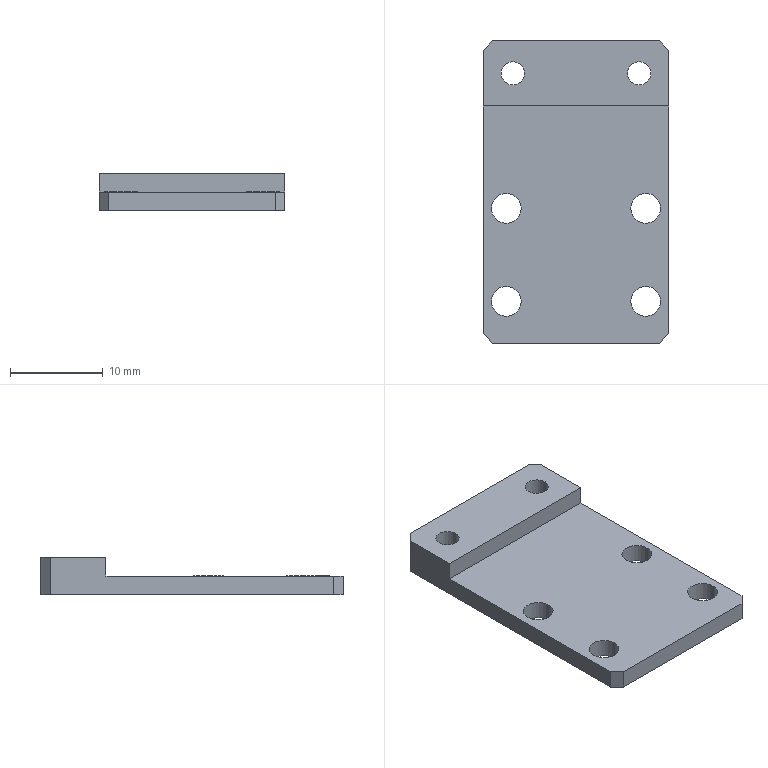Part | STEP file | 11-FG-B08011 | 1 solid | 24 faces | box 20 x 32.5 x 4 mm | volume 1470 mm3 | cylinder 12 | plane 12 | commonest cylinder face diameters 3.2 x8 2.5 x4
STEP:
#1=CARTESIAN_POINT('',(5.55,12.75,4.));
#2=VERTEX_POINT('',#1);
#3=CARTESIAN_POINT('',(8.05,12.75,4.));
#4=VERTEX_POINT('',#3);
#5=CARTESIAN_POINT('',(6.8,12.75,4.));
#6=DIRECTION('',(0.,0.,1.));
#7=DIRECTION('',(1.,0.,0.));
#8=AXIS2_PLACEMENT_3D('',#5,#6,#7);
#9=CIRCLE('',#8,1.25);
#10=EDGE_CURVE('',#2,#4,#9,.T.);
#11=ORIENTED_EDGE('',*,*,#10,.T.);
#12=CARTESIAN_POINT('',(8.05,12.75,0.));
#13=VERTEX_POINT('',#12);
#14=CARTESIAN_POINT('',(8.05,12.75,0.));
#15=DIRECTION('',(0.,0.,-1.));
#16=VECTOR('',#15,1000.);
#17=LINE('',#14,#16);
#18=EDGE_CURVE('',#4,#13,#17,.T.);
#19=ORIENTED_EDGE('',*,*,#18,.T.);
#20=CARTESIAN_POINT('',(5.55,12.75,0.));
#21=VERTEX_POINT('',#20);
#22=CARTESIAN_POINT('',(6.8,12.75,0.));
#23=DIRECTION('',(0.,0.,-1.));
#24=DIRECTION('',(-1.,0.,0.));
#25=AXIS2_PLACEMENT_3D('',#22,#23,#24);
#26=CIRCLE('',#25,1.25);
#27=EDGE_CURVE('',#13,#21,#26,.T.);
#28=ORIENTED_EDGE('',*,*,#27,.T.);
#29=CARTESIAN_POINT('',(5.55,12.75,0.));
#30=DIRECTION('',(0.,0.,-1.));
#31=VECTOR('',#30,1000.);
#32=LINE('',#29,#31);
#33=EDGE_CURVE('',#2,#21,#32,.T.);
#34=ORIENTED_EDGE('',*,*,#33,.F.);
#35=EDGE_LOOP('',(#11,#19,#28,#34));
#36=FACE_OUTER_BOUND('',#35,.T.);
#37=CARTESIAN_POINT('',(6.8,12.75,0.));
#38=DIRECTION('',(0.,0.,-1.));
#39=DIRECTION('',(-1.,0.,0.));
#40=AXIS2_PLACEMENT_3D('',#37,#38,#39);
#41=CYLINDRICAL_SURFACE('',#40,1.25);
#42=ADVANCED_FACE('',(#36),#41,.F.);
#43=CARTESIAN_POINT('',(-8.05,12.75,4.));
#44=VERTEX_POINT('',#43);
#45=CARTESIAN_POINT('',(-5.55,12.75,4.));
#46=VERTEX_POINT('',#45);
#47=CARTESIAN_POINT('',(-6.8,12.75,4.));
#48=DIRECTION('',(0.,0.,1.));
#49=DIRECTION('',(1.,0.,0.));
#50=AXIS2_PLACEMENT_3D('',#47,#48,#49);
#51=CIRCLE('',#50,1.25);
#52=EDGE_CURVE('',#44,#46,#51,.T.);
#53=ORIENTED_EDGE('',*,*,#52,.T.);
#54=CARTESIAN_POINT('',(-5.55,12.75,0.));
#55=VERTEX_POINT('',#54);
#56=CARTESIAN_POINT('',(-5.55,12.75,0.));
#57=DIRECTION('',(0.,0.,-1.));
#58=VECTOR('',#57,1000.);
#59=LINE('',#56,#58);
#60=EDGE_CURVE('',#46,#55,#59,.T.);
#61=ORIENTED_EDGE('',*,*,#60,.T.);
#62=CARTESIAN_POINT('',(-8.05,12.75,0.));
#63=VERTEX_POINT('',#62);
#64=CARTESIAN_POINT('',(-6.8,12.75,0.));
#65=DIRECTION('',(0.,0.,-1.));
#66=DIRECTION('',(-1.,0.,0.));
#67=AXIS2_PLACEMENT_3D('',#64,#65,#66);
#68=CIRCLE('',#67,1.25);
#69=EDGE_CURVE('',#55,#63,#68,.T.);
#70=ORIENTED_EDGE('',*,*,#69,.T.);
#71=CARTESIAN_POINT('',(-8.05,12.75,0.));
#72=DIRECTION('',(0.,0.,-1.));
#73=VECTOR('',#72,1000.);
#74=LINE('',#71,#73);
#75=EDGE_CURVE('',#44,#63,#74,.T.);
#76=ORIENTED_EDGE('',*,*,#75,.F.);
#77=EDGE_LOOP('',(#53,#61,#70,#76));
#78=FACE_OUTER_BOUND('',#77,.T.);
#79=CARTESIAN_POINT('',(-6.8,12.75,0.));
#80=DIRECTION('',(0.,0.,-1.));
#81=DIRECTION('',(-1.,0.,0.));
#82=AXIS2_PLACEMENT_3D('',#79,#80,#81);
#83=CYLINDRICAL_SURFACE('',#82,1.25);
#84=ADVANCED_FACE('',(#78),#83,.F.);
#85=CARTESIAN_POINT('',(5.9,-1.75,2.));
#86=VERTEX_POINT('',#85);
#87=CARTESIAN_POINT('',(9.1,-1.75,2.));
#88=VERTEX_POINT('',#87);
#89=CARTESIAN_POINT('',(7.5,-1.75,2.));
#90=DIRECTION('',(0.,0.,1.));
#91=DIRECTION('',(1.,0.,0.));
#92=AXIS2_PLACEMENT_3D('',#89,#90,#91);
#93=CIRCLE('',#92,1.6);
#94=EDGE_CURVE('',#86,#88,#93,.T.);
#95=ORIENTED_EDGE('',*,*,#94,.T.);
#96=CARTESIAN_POINT('',(9.1,-1.75,0.));
#97=VERTEX_POINT('',#96);
#98=CARTESIAN_POINT('',(9.1,-1.75,24.));
#99=DIRECTION('',(0.,0.,-1.));
#100=VECTOR('',#99,1000.);
#101=LINE('',#98,#100);
#102=EDGE_CURVE('',#88,#97,#101,.T.);
#103=ORIENTED_EDGE('',*,*,#102,.T.);
#104=CARTESIAN_POINT('',(5.9,-1.75,0.));
#105=VERTEX_POINT('',#104);
#106=CARTESIAN_POINT('',(7.5,-1.75,0.));
#107=DIRECTION('',(0.,0.,-1.));
#108=DIRECTION('',(-1.,0.,0.));
#109=AXIS2_PLACEMENT_3D('',#106,#107,#108);
#110=CIRCLE('',#109,1.6);
#111=EDGE_CURVE('',#97,#105,#110,.T.);
#112=ORIENTED_EDGE('',*,*,#111,.T.);
#113=CARTESIAN_POINT('',(5.9,-1.75,24.));
#114=DIRECTION('',(0.,0.,-1.));
#115=VECTOR('',#114,1000.);
#116=LINE('',#113,#115);
#117=EDGE_CURVE('',#86,#105,#116,.T.);
#118=ORIENTED_EDGE('',*,*,#117,.F.);
#119=EDGE_LOOP('',(#95,#103,#112,#118));
#120=FACE_OUTER_BOUND('',#119,.T.);
#121=CARTESIAN_POINT('',(7.5,-1.75,24.));
#122=DIRECTION('',(0.,0.,-1.));
#123=DIRECTION('',(-1.,0.,0.));
#124=AXIS2_PLACEMENT_3D('',#121,#122,#123);
#125=CYLINDRICAL_SURFACE('',#124,1.6);
#126=ADVANCED_FACE('',(#120),#125,.F.);
#127=CARTESIAN_POINT('',(-9.1,-1.75,2.));
#128=VERTEX_POINT('',#127);
#129=CARTESIAN_POINT('',(-5.9,-1.75,2.));
#130=VERTEX_POINT('',#129);
#131=CARTESIAN_POINT('',(-7.5,-1.75,2.));
#132=DIRECTION('',(0.,0.,1.));
#133=DIRECTION('',(1.,0.,0.));
#134=AXIS2_PLACEMENT_3D('',#131,#132,#133);
#135=CIRCLE('',#134,1.6);
#136=EDGE_CURVE('',#128,#130,#135,.T.);
#137=ORIENTED_EDGE('',*,*,#136,.T.);
#138=CARTESIAN_POINT('',(-5.9,-1.75,0.));
#139=VERTEX_POINT('',#138);
#140=CARTESIAN_POINT('',(-5.9,-1.75,24.));
#141=DIRECTION('',(0.,0.,-1.));
#142=VECTOR('',#141,1000.);
#143=LINE('',#140,#142);
#144=EDGE_CURVE('',#130,#139,#143,.T.);
#145=ORIENTED_EDGE('',*,*,#144,.T.);
#146=CARTESIAN_POINT('',(-9.1,-1.75,0.));
#147=VERTEX_POINT('',#146);
#148=CARTESIAN_POINT('',(-7.5,-1.75,0.));
#149=DIRECTION('',(0.,0.,-1.));
#150=DIRECTION('',(-1.,0.,0.));
#151=AXIS2_PLACEMENT_3D('',#148,#149,#150);
#152=CIRCLE('',#151,1.6);
#153=EDGE_CURVE('',#139,#147,#152,.T.);
#154=ORIENTED_EDGE('',*,*,#153,.T.);
#155=CARTESIAN_POINT('',(-9.1,-1.75,24.));
#156=DIRECTION('',(0.,0.,-1.));
#157=VECTOR('',#156,1000.);
#158=LINE('',#155,#157);
#159=EDGE_CURVE('',#128,#147,#158,.T.);
#160=ORIENTED_EDGE('',*,*,#159,.F.);
#161=EDGE_LOOP('',(#137,#145,#154,#160));
#162=FACE_OUTER_BOUND('',#161,.T.);
#163=CARTESIAN_POINT('',(-7.5,-1.75,24.));
#164=DIRECTION('',(0.,0.,-1.));
#165=DIRECTION('',(-1.,0.,0.));
#166=AXIS2_PLACEMENT_3D('',#163,#164,#165);
#167=CYLINDRICAL_SURFACE('',#166,1.6);
#168=ADVANCED_FACE('',(#162),#167,.F.);
#169=CARTESIAN_POINT('',(-9.1,-11.75,2.));
#170=VERTEX_POINT('',#169);
#171=CARTESIAN_POINT('',(-5.9,-11.75,2.));
#172=VERTEX_POINT('',#171);
#173=CARTESIAN_POINT('',(-7.5,-11.75,2.));
#174=DIRECTION('',(0.,0.,1.));
#175=DIRECTION('',(1.,0.,0.));
#176=AXIS2_PLACEMENT_3D('',#173,#174,#175);
#177=CIRCLE('',#176,1.6);
#178=EDGE_CURVE('',#170,#172,#177,.T.);
#179=ORIENTED_EDGE('',*,*,#178,.T.);
#180=CARTESIAN_POINT('',(-5.9,-11.75,0.));
#181=VERTEX_POINT('',#180);
#182=CARTESIAN_POINT('',(-5.9,-11.75,24.));
#183=DIRECTION('',(0.,0.,-1.));
#184=VECTOR('',#183,1000.);
#185=LINE('',#182,#184);
#186=EDGE_CURVE('',#172,#181,#185,.T.);
#187=ORIENTED_EDGE('',*,*,#186,.T.);
#188=CARTESIAN_POINT('',(-9.1,-11.75,0.));
#189=VERTEX_POINT('',#188);
#190=CARTESIAN_POINT('',(-7.5,-11.75,0.));
#191=DIRECTION('',(0.,0.,-1.));
#192=DIRECTION('',(-1.,0.,0.));
#193=AXIS2_PLACEMENT_3D('',#190,#191,#192);
#194=CIRCLE('',#193,1.6);
#195=EDGE_CURVE('',#181,#189,#194,.T.);
#196=ORIENTED_EDGE('',*,*,#195,.T.);
#197=CARTESIAN_POINT('',(-9.1,-11.75,24.));
#198=DIRECTION('',(0.,0.,-1.));
#199=VECTOR('',#198,1000.);
#200=LINE('',#197,#199);
#201=EDGE_CURVE('',#170,#189,#200,.T.);
#202=ORIENTED_EDGE('',*,*,#201,.F.);
#203=EDGE_LOOP('',(#179,#187,#196,#202));
#204=FACE_OUTER_BOUND('',#203,.T.);
#205=CARTESIAN_POINT('',(-7.5,-11.75,24.));
#206=DIRECTION('',(0.,0.,-1.));
#207=DIRECTION('',(-1.,0.,0.));
#208=AXIS2_PLACEMENT_3D('',#205,#206,#207);
#209=CYLINDRICAL_SURFACE('',#208,1.6);
#210=ADVANCED_FACE('',(#204),#209,.F.);
#211=CARTESIAN_POINT('',(5.9,-11.75,2.));
#212=VERTEX_POINT('',#211);
#213=CARTESIAN_POINT('',(9.1,-11.75,2.));
#214=VERTEX_POINT('',#213);
#215=CARTESIAN_POINT('',(7.5,-11.75,2.));
#216=DIRECTION('',(0.,0.,1.));
#217=DIRECTION('',(1.,0.,0.));
#218=AXIS2_PLACEMENT_3D('',#215,#216,#217);
#219=CIRCLE('',#218,1.6);
#220=EDGE_CURVE('',#212,#214,#219,.T.);
#221=ORIENTED_EDGE('',*,*,#220,.T.);
#222=CARTESIAN_POINT('',(9.1,-11.75,0.));
#223=VERTEX_POINT('',#222);
#224=CARTESIAN_POINT('',(9.1,-11.75,24.));
#225=DIRECTION('',(0.,0.,-1.));
#226=VECTOR('',#225,1000.);
#227=LINE('',#224,#226);
#228=EDGE_CURVE('',#214,#223,#227,.T.);
#229=ORIENTED_EDGE('',*,*,#228,.T.);
#230=CARTESIAN_POINT('',(5.9,-11.75,0.));
#231=VERTEX_POINT('',#230);
#232=CARTESIAN_POINT('',(7.5,-11.75,0.));
#233=DIRECTION('',(0.,0.,-1.));
#234=DIRECTION('',(-1.,0.,0.));
#235=AXIS2_PLACEMENT_3D('',#232,#233,#234);
#236=CIRCLE('',#235,1.6);
#237=EDGE_CURVE('',#223,#231,#236,.T.);
#238=ORIENTED_EDGE('',*,*,#237,.T.);
#239=CARTESIAN_POINT('',(5.9,-11.75,24.));
#240=DIRECTION('',(0.,0.,-1.));
#241=VECTOR('',#240,1000.);
#242=LINE('',#239,#241);
#243=EDGE_CURVE('',#212,#231,#242,.T.);
#244=ORIENTED_EDGE('',*,*,#243,.F.);
#245=EDGE_LOOP('',(#221,#229,#238,#244));
#246=FACE_OUTER_BOUND('',#245,.T.);
#247=CARTESIAN_POINT('',(7.5,-11.75,24.));
#248=DIRECTION('',(0.,0.,-1.));
#249=DIRECTION('',(-1.,0.,0.));
#250=AXIS2_PLACEMENT_3D('',#247,#248,#249);
#251=CYLINDRICAL_SURFACE('',#250,1.6);
#252=ADVANCED_FACE('',(#246),#251,.F.);
#253=CARTESIAN_POINT('',(10.,-15.25,2.));
#254=VERTEX_POINT('',#253);
#255=CARTESIAN_POINT('',(10.,9.25,2.));
#256=VERTEX_POINT('',#255);
#257=CARTESIAN_POINT('',(10.,16.25,2.));
#258=DIRECTION('',(0.,1.,0.));
#259=VECTOR('',#258,1000.);
#260=LINE('',#257,#259);
#261=EDGE_CURVE('',#254,#256,#260,.T.);
#262=ORIENTED_EDGE('',*,*,#261,.F.);
#263=CARTESIAN_POINT('',(10.,-15.25,0.));
#264=VERTEX_POINT('',#263);
#265=CARTESIAN_POINT('',(10.,-15.25,2.));
#266=DIRECTION('',(0.,0.,-1.));
#267=VECTOR('',#266,1000.);
#268=LINE('',#265,#267);
#269=EDGE_CURVE('',#254,#264,#268,.T.);
#270=ORIENTED_EDGE('',*,*,#269,.T.);
#271=CARTESIAN_POINT('',(10.,15.25,0.));
#272=VERTEX_POINT('',#271);
#273=CARTESIAN_POINT('',(10.,16.25,0.));
#274=DIRECTION('',(0.,1.,0.));
#275=VECTOR('',#274,1000.);
#276=LINE('',#273,#275);
#277=EDGE_CURVE('',#264,#272,#276,.T.);
#278=ORIENTED_EDGE('',*,*,#277,.T.);
#279=CARTESIAN_POINT('',(10.,15.25,4.));
#280=VERTEX_POINT('',#279);
#281=CARTESIAN_POINT('',(10.,15.25,2.));
#282=DIRECTION('',(0.,0.,1.));
#283=VECTOR('',#282,1000.);
#284=LINE('',#281,#283);
#285=EDGE_CURVE('',#272,#280,#284,.T.);
#286=ORIENTED_EDGE('',*,*,#285,.T.);
#287=CARTESIAN_POINT('',(10.,9.25,4.));
#288=VERTEX_POINT('',#287);
#289=CARTESIAN_POINT('',(10.,16.25,4.));
#290=DIRECTION('',(0.,1.,0.));
#291=VECTOR('',#290,1000.);
#292=LINE('',#289,#291);
#293=EDGE_CURVE('',#288,#280,#292,.T.);
#294=ORIENTED_EDGE('',*,*,#293,.F.);
#295=CARTESIAN_POINT('',(10.,9.25,4.));
#296=DIRECTION('',(0.,0.,-1.));
#297=VECTOR('',#296,1000.);
#298=LINE('',#295,#297);
#299=EDGE_CURVE('',#288,#256,#298,.T.);
#300=ORIENTED_EDGE('',*,*,#299,.T.);
#301=EDGE_LOOP('',(#262,#270,#278,#286,#294,#300));
#302=FACE_OUTER_BOUND('',#301,.T.);
#303=CARTESIAN_POINT('',(10.,16.25,2.));
#304=DIRECTION('',(-1.,0.,0.));
#305=DIRECTION('',(0.,-1.,0.));
#306=AXIS2_PLACEMENT_3D('',#303,#304,#305);
#307=PLANE('',#306);
#308=ADVANCED_FACE('',(#302),#307,.F.);
#309=CARTESIAN_POINT('',(9.,16.25,0.));
#310=VERTEX_POINT('',#309);
#311=CARTESIAN_POINT('',(-9.,16.25,0.));
#312=VERTEX_POINT('',#311);
#313=CARTESIAN_POINT('',(-10.,16.25,0.));
#314=DIRECTION('',(-1.,0.,0.));
#315=VECTOR('',#314,1000.);
#316=LINE('',#313,#315);
#317=EDGE_CURVE('',#310,#312,#316,.T.);
#318=ORIENTED_EDGE('',*,*,#317,.T.);
#319=CARTESIAN_POINT('',(-9.,16.25,4.));
#320=VERTEX_POINT('',#319);
#321=CARTESIAN_POINT('',(-9.,16.25,2.));
#322=DIRECTION('',(0.,0.,1.));
#323=VECTOR('',#322,1000.);
#324=LINE('',#321,#323);
#325=EDGE_CURVE('',#312,#320,#324,.T.);
#326=ORIENTED_EDGE('',*,*,#325,.T.);
#327=CARTESIAN_POINT('',(9.,16.25,4.));
#328=VERTEX_POINT('',#327);
#329=CARTESIAN_POINT('',(-10.,16.25,4.));
#330=DIRECTION('',(-1.,0.,0.));
#331=VECTOR('',#330,1000.);
#332=LINE('',#329,#331);
#333=EDGE_CURVE('',#328,#320,#332,.T.);
#334=ORIENTED_EDGE('',*,*,#333,.F.);
#335=CARTESIAN_POINT('',(9.,16.25,2.));
#336=DIRECTION('',(0.,0.,-1.));
#337=VECTOR('',#336,1000.);
#338=LINE('',#335,#337);
#339=EDGE_CURVE('',#328,#310,#338,.T.);
#340=ORIENTED_EDGE('',*,*,#339,.T.);
#341=EDGE_LOOP('',(#318,#326,#334,#340));
#342=FACE_OUTER_BOUND('',#341,.T.);
#343=CARTESIAN_POINT('',(-10.,16.25,2.));
#344=DIRECTION('',(0.,-1.,0.));
#345=DIRECTION('',(0.,0.,-1.));
#346=AXIS2_PLACEMENT_3D('',#343,#344,#345);
#347=PLANE('',#346);
#348=ADVANCED_FACE('',(#342),#347,.F.);
#349=CARTESIAN_POINT('',(-10.,15.25,0.));
#350=VERTEX_POINT('',#349);
#351=CARTESIAN_POINT('',(-10.,-15.25,0.));
#352=VERTEX_POINT('',#351);
#353=CARTESIAN_POINT('',(-10.,16.25,0.));
#354=DIRECTION('',(0.,-1.,0.));
#355=VECTOR('',#354,1000.);
#356=LINE('',#353,#355);
#357=EDGE_CURVE('',#350,#352,#356,.T.);
#358=ORIENTED_EDGE('',*,*,#357,.T.);
#359=CARTESIAN_POINT('',(-10.,-15.25,2.));
#360=VERTEX_POINT('',#359);
#361=CARTESIAN_POINT('',(-10.,-15.25,2.));
#362=DIRECTION('',(0.,0.,1.));
#363=VECTOR('',#362,1000.);
#364=LINE('',#361,#363);
#365=EDGE_CURVE('',#352,#360,#364,.T.);
#366=ORIENTED_EDGE('',*,*,#365,.T.);
#367=CARTESIAN_POINT('',(-10.,9.25,2.));
#368=VERTEX_POINT('',#367);
#369=CARTESIAN_POINT('',(-10.,16.25,2.));
#370=DIRECTION('',(0.,-1.,0.));
#371=VECTOR('',#370,1000.);
#372=LINE('',#369,#371);
#373=EDGE_CURVE('',#368,#360,#372,.T.);
#374=ORIENTED_EDGE('',*,*,#373,.F.);
#375=CARTESIAN_POINT('',(-10.,9.25,4.));
#376=VERTEX_POINT('',#375);
#377=CARTESIAN_POINT('',(-10.,9.25,4.));
#378=DIRECTION('',(0.,0.,-1.));
#379=VECTOR('',#378,1000.);
#380=LINE('',#377,#379);
#381=EDGE_CURVE('',#376,#368,#380,.T.);
#382=ORIENTED_EDGE('',*,*,#381,.F.);
#383=CARTESIAN_POINT('',(-10.,15.25,4.));
#384=VERTEX_POINT('',#383);
#385=CARTESIAN_POINT('',(-10.,16.25,4.));
#386=DIRECTION('',(0.,-1.,0.));
#387=VECTOR('',#386,1000.);
#388=LINE('',#385,#387);
#389=EDGE_CURVE('',#384,#376,#388,.T.);
#390=ORIENTED_EDGE('',*,*,#389,.F.);
#391=CARTESIAN_POINT('',(-10.,15.25,2.));
#392=DIRECTION('',(0.,0.,-1.));
#393=VECTOR('',#392,1000.);
#394=LINE('',#391,#393);
#395=EDGE_CURVE('',#384,#350,#394,.T.);
#396=ORIENTED_EDGE('',*,*,#395,.T.);
#397=EDGE_LOOP('',(#358,#366,#374,#382,#390,#396));
#398=FACE_OUTER_BOUND('',#397,.T.);
#399=CARTESIAN_POINT('',(-10.,16.25,2.));
#400=DIRECTION('',(1.,0.,0.));
#401=DIRECTION('',(0.,1.,0.));
#402=AXIS2_PLACEMENT_3D('',#399,#400,#401);
#403=PLANE('',#402);
#404=ADVANCED_FACE('',(#398),#403,.F.);
#405=CARTESIAN_POINT('',(-9.,-16.25,0.));
#406=VERTEX_POINT('',#405);
#407=CARTESIAN_POINT('',(9.,-16.25,0.));
#408=VERTEX_POINT('',#407);
#409=CARTESIAN_POINT('',(-10.,-16.25,0.));
#410=DIRECTION('',(1.,0.,0.));
#411=VECTOR('',#410,1000.);
#412=LINE('',#409,#411);
#413=EDGE_CURVE('',#406,#408,#412,.T.);
#414=ORIENTED_EDGE('',*,*,#413,.T.);
#415=CARTESIAN_POINT('',(9.,-16.25,2.));
#416=VERTEX_POINT('',#415);
#417=CARTESIAN_POINT('',(9.,-16.25,2.));
#418=DIRECTION('',(0.,0.,1.));
#419=VECTOR('',#418,1000.);
#420=LINE('',#417,#419);
#421=EDGE_CURVE('',#408,#416,#420,.T.);
#422=ORIENTED_EDGE('',*,*,#421,.T.);
#423=CARTESIAN_POINT('',(-9.,-16.25,2.));
#424=VERTEX_POINT('',#423);
#425=CARTESIAN_POINT('',(-10.,-16.25,2.));
#426=DIRECTION('',(1.,0.,0.));
#427=VECTOR('',#426,1000.);
#428=LINE('',#425,#427);
#429=EDGE_CURVE('',#424,#416,#428,.T.);
#430=ORIENTED_EDGE('',*,*,#429,.F.);
#431=CARTESIAN_POINT('',(-9.,-16.25,2.));
#432=DIRECTION('',(0.,0.,-1.));
#433=VECTOR('',#432,1000.);
#434=LINE('',#431,#433);
#435=EDGE_CURVE('',#424,#406,#434,.T.);
#436=ORIENTED_EDGE('',*,*,#435,.T.);
#437=EDGE_LOOP('',(#414,#422,#430,#436));
#438=FACE_OUTER_BOUND('',#437,.T.);
#439=CARTESIAN_POINT('',(-10.,-16.25,2.));
#440=DIRECTION('',(0.,1.,0.));
#441=DIRECTION('',(0.,0.,1.));
#442=AXIS2_PLACEMENT_3D('',#439,#440,#441);
#443=PLANE('',#442);
#444=ADVANCED_FACE('',(#438),#443,.F.);
#445=ORIENTED_EDGE('',*,*,#429,.T.);
#446=CARTESIAN_POINT('',(12.625,-12.625,2.));
#447=DIRECTION('',(0.7071,0.7071,0.));
#448=VECTOR('',#447,1000.);
#449=LINE('',#446,#448);
#450=EDGE_CURVE('',#416,#254,#449,.T.);
#451=ORIENTED_EDGE('',*,*,#450,.T.);
#452=ORIENTED_EDGE('',*,*,#261,.T.);
#453=CARTESIAN_POINT('',(-10.,9.25,2.));
#454=DIRECTION('',(1.,0.,0.));
#455=VECTOR('',#454,1000.);
#456=LINE('',#453,#455);
#457=EDGE_CURVE('',#368,#256,#456,.T.);
#458=ORIENTED_EDGE('',*,*,#457,.F.);
#459=ORIENTED_EDGE('',*,*,#373,.T.);
#460=CARTESIAN_POINT('',(-12.625,-12.625,2.));
#461=DIRECTION('',(0.7071,-0.7071,0.));
#462=VECTOR('',#461,1000.);
#463=LINE('',#460,#462);
#464=EDGE_CURVE('',#360,#424,#463,.T.);
#465=ORIENTED_EDGE('',*,*,#464,.T.);
#466=EDGE_LOOP('',(#445,#451,#452,#458,#459,#465));
#467=FACE_OUTER_BOUND('',#466,.T.);
#468=ORIENTED_EDGE('',*,*,#94,.F.);
#469=CARTESIAN_POINT('',(7.5,-1.75,2.));
#470=DIRECTION('',(0.,0.,1.));
#471=DIRECTION('',(1.,0.,0.));
#472=AXIS2_PLACEMENT_3D('',#469,#470,#471);
#473=CIRCLE('',#472,1.6);
#474=EDGE_CURVE('',#88,#86,#473,.T.);
#475=ORIENTED_EDGE('',*,*,#474,.F.);
#476=EDGE_LOOP('',(#468,#475));
#477=FACE_BOUND('',#476,.T.);
#478=ORIENTED_EDGE('',*,*,#136,.F.);
#479=CARTESIAN_POINT('',(-7.5,-1.75,2.));
#480=DIRECTION('',(0.,0.,1.));
#481=DIRECTION('',(1.,0.,0.));
#482=AXIS2_PLACEMENT_3D('',#479,#480,#481);
#483=CIRCLE('',#482,1.6);
#484=EDGE_CURVE('',#130,#128,#483,.T.);
#485=ORIENTED_EDGE('',*,*,#484,.F.);
#486=EDGE_LOOP('',(#478,#485));
#487=FACE_BOUND('',#486,.T.);
#488=ORIENTED_EDGE('',*,*,#178,.F.);
#489=CARTESIAN_POINT('',(-7.5,-11.75,2.));
#490=DIRECTION('',(0.,0.,1.));
#491=DIRECTION('',(1.,0.,0.));
#492=AXIS2_PLACEMENT_3D('',#489,#490,#491);
#493=CIRCLE('',#492,1.6);
#494=EDGE_CURVE('',#172,#170,#493,.T.);
#495=ORIENTED_EDGE('',*,*,#494,.F.);
#496=EDGE_LOOP('',(#488,#495));
#497=FACE_BOUND('',#496,.T.);
#498=ORIENTED_EDGE('',*,*,#220,.F.);
#499=CARTESIAN_POINT('',(7.5,-11.75,2.));
#500=DIRECTION('',(0.,0.,1.));
#501=DIRECTION('',(1.,0.,0.));
#502=AXIS2_PLACEMENT_3D('',#499,#500,#501);
#503=CIRCLE('',#502,1.6);
#504=EDGE_CURVE('',#214,#212,#503,.T.);
#505=ORIENTED_EDGE('',*,*,#504,.F.);
#506=EDGE_LOOP('',(#498,#505));
#507=FACE_BOUND('',#506,.T.);
#508=CARTESIAN_POINT('',(0.,0.,2.));
#509=DIRECTION('',(0.,0.,1.));
#510=DIRECTION('',(1.,0.,0.));
#511=AXIS2_PLACEMENT_3D('',#508,#509,#510);
#512=PLANE('',#511);
#513=ADVANCED_FACE('',(#467,#477,#487,#497,#507),#512,.T.);
#514=CARTESIAN_POINT('',(6.8,12.75,0.));
#515=DIRECTION('',(0.,0.,-1.));
#516=DIRECTION('',(-1.,0.,0.));
#517=AXIS2_PLACEMENT_3D('',#514,#515,#516);
#518=CIRCLE('',#517,1.25);
#519=EDGE_CURVE('',#21,#13,#518,.T.);
#520=ORIENTED_EDGE('',*,*,#519,.F.);
#521=ORIENTED_EDGE('',*,*,#27,.F.);
#522=EDGE_LOOP('',(#520,#521));
#523=FACE_BOUND('',#522,.T.);
#524=CARTESIAN_POINT('',(-6.8,12.75,0.));
#525=DIRECTION('',(0.,0.,-1.));
#526=DIRECTION('',(-1.,0.,0.));
#527=AXIS2_PLACEMENT_3D('',#524,#525,#526);
#528=CIRCLE('',#527,1.25);
#529=EDGE_CURVE('',#63,#55,#528,.T.);
#530=ORIENTED_EDGE('',*,*,#529,.F.);
#531=ORIENTED_EDGE('',*,*,#69,.F.);
#532=EDGE_LOOP('',(#530,#531));
#533=FACE_BOUND('',#532,.T.);
#534=CARTESIAN_POINT('',(7.5,-1.75,0.));
#535=DIRECTION('',(0.,0.,-1.));
#536=DIRECTION('',(-1.,0.,0.));
#537=AXIS2_PLACEMENT_3D('',#534,#535,#536);
#538=CIRCLE('',#537,1.6);
#539=EDGE_CURVE('',#105,#97,#538,.T.);
#540=ORIENTED_EDGE('',*,*,#539,.F.);
#541=ORIENTED_EDGE('',*,*,#111,.F.);
#542=EDGE_LOOP('',(#540,#541));
#543=FACE_BOUND('',#542,.T.);
#544=CARTESIAN_POINT('',(-7.5,-1.75,0.));
#545=DIRECTION('',(0.,0.,-1.));
#546=DIRECTION('',(-1.,0.,0.));
#547=AXIS2_PLACEMENT_3D('',#544,#545,#546);
#548=CIRCLE('',#547,1.6);
#549=EDGE_CURVE('',#147,#139,#548,.T.);
#550=ORIENTED_EDGE('',*,*,#549,.F.);
#551=ORIENTED_EDGE('',*,*,#153,.F.);
#552=EDGE_LOOP('',(#550,#551));
#553=FACE_BOUND('',#552,.T.);
#554=CARTESIAN_POINT('',(-7.5,-11.75,0.));
#555=DIRECTION('',(0.,0.,-1.));
#556=DIRECTION('',(-1.,0.,0.));
#557=AXIS2_PLACEMENT_3D('',#554,#555,#556);
#558=CIRCLE('',#557,1.6);
#559=EDGE_CURVE('',#189,#181,#558,.T.);
#560=ORIENTED_EDGE('',*,*,#559,.F.);
#561=ORIENTED_EDGE('',*,*,#195,.F.);
#562=EDGE_LOOP('',(#560,#561));
#563=FACE_BOUND('',#562,.T.);
#564=CARTESIAN_POINT('',(7.5,-11.75,0.));
#565=DIRECTION('',(0.,0.,-1.));
#566=DIRECTION('',(-1.,0.,0.));
#567=AXIS2_PLACEMENT_3D('',#564,#565,#566);
#568=CIRCLE('',#567,1.6);
#569=EDGE_CURVE('',#231,#223,#568,.T.);
#570=ORIENTED_EDGE('',*,*,#569,.F.);
#571=ORIENTED_EDGE('',*,*,#237,.F.);
#572=EDGE_LOOP('',(#570,#571));
#573=FACE_BOUND('',#572,.T.);
#574=ORIENTED_EDGE('',*,*,#277,.F.);
#575=CARTESIAN_POINT('',(10.,-15.25,0.));
#576=DIRECTION('',(-0.7071,-0.7071,0.));
#577=VECTOR('',#576,1000.);
#578=LINE('',#575,#577);
#579=EDGE_CURVE('',#264,#408,#578,.T.);
#580=ORIENTED_EDGE('',*,*,#579,.T.);
#581=ORIENTED_EDGE('',*,*,#413,.F.);
#582=CARTESIAN_POINT('',(-9.,-16.25,0.));
#583=DIRECTION('',(-0.7071,0.7071,0.));
#584=VECTOR('',#583,1000.);
#585=LINE('',#582,#584);
#586=EDGE_CURVE('',#406,#352,#585,.T.);
#587=ORIENTED_EDGE('',*,*,#586,.T.);
#588=ORIENTED_EDGE('',*,*,#357,.F.);
#589=CARTESIAN_POINT('',(-10.,15.25,0.));
#590=DIRECTION('',(0.7071,0.7071,0.));
#591=VECTOR('',#590,1000.);
#592=LINE('',#589,#591);
#593=EDGE_CURVE('',#350,#312,#592,.T.);
#594=ORIENTED_EDGE('',*,*,#593,.T.);
#595=ORIENTED_EDGE('',*,*,#317,.F.);
#596=CARTESIAN_POINT('',(9.,16.25,0.));
#597=DIRECTION('',(0.7071,-0.7071,0.));
#598=VECTOR('',#597,1000.);
#599=LINE('',#596,#598);
#600=EDGE_CURVE('',#310,#272,#599,.T.);
#601=ORIENTED_EDGE('',*,*,#600,.T.);
#602=EDGE_LOOP('',(#574,#580,#581,#587,#588,#594,#595,#601));
#603=FACE_OUTER_BOUND('',#602,.T.);
#604=CARTESIAN_POINT('',(0.,0.,0.));
#605=DIRECTION('',(0.,0.,1.));
#606=DIRECTION('',(1.,0.,0.));
#607=AXIS2_PLACEMENT_3D('',#604,#605,#606);
#608=PLANE('',#607);
#609=ADVANCED_FACE('',(#523,#533,#543,#553,#563,#573,#603),#608,.F.);
#610=ORIENTED_EDGE('',*,*,#228,.F.);
#611=ORIENTED_EDGE('',*,*,#504,.T.);
#612=ORIENTED_EDGE('',*,*,#243,.T.);
#613=ORIENTED_EDGE('',*,*,#569,.T.);
#614=EDGE_LOOP('',(#610,#611,#612,#613));
#615=FACE_OUTER_BOUND('',#614,.T.);
#616=CARTESIAN_POINT('',(7.5,-11.75,24.));
#617=DIRECTION('',(0.,0.,-1.));
#618=DIRECTION('',(-1.,0.,0.));
#619=AXIS2_PLACEMENT_3D('',#616,#617,#618);
#620=CYLINDRICAL_SURFACE('',#619,1.6);
#621=ADVANCED_FACE('',(#615),#620,.F.);
#622=ORIENTED_EDGE('',*,*,#186,.F.);
#623=ORIENTED_EDGE('',*,*,#494,.T.);
#624=ORIENTED_EDGE('',*,*,#201,.T.);
#625=ORIENTED_EDGE('',*,*,#559,.T.);
#626=EDGE_LOOP('',(#622,#623,#624,#625));
#627=FACE_OUTER_BOUND('',#626,.T.);
#628=CARTESIAN_POINT('',(-7.5,-11.75,24.));
#629=DIRECTION('',(0.,0.,-1.));
#630=DIRECTION('',(-1.,0.,0.));
#631=AXIS2_PLACEMENT_3D('',#628,#629,#630);
#632=CYLINDRICAL_SURFACE('',#631,1.6);
#633=ADVANCED_FACE('',(#627),#632,.F.);
#634=ORIENTED_EDGE('',*,*,#144,.F.);
#635=ORIENTED_EDGE('',*,*,#484,.T.);
#636=ORIENTED_EDGE('',*,*,#159,.T.);
#637=ORIENTED_EDGE('',*,*,#549,.T.);
#638=EDGE_LOOP('',(#634,#635,#636,#637));
#639=FACE_OUTER_BOUND('',#638,.T.);
#640=CARTESIAN_POINT('',(-7.5,-1.75,24.));
#641=DIRECTION('',(0.,0.,-1.));
#642=DIRECTION('',(-1.,0.,0.));
#643=AXIS2_PLACEMENT_3D('',#640,#641,#642);
#644=CYLINDRICAL_SURFACE('',#643,1.6);
#645=ADVANCED_FACE('',(#639),#644,.F.);
#646=ORIENTED_EDGE('',*,*,#102,.F.);
#647=ORIENTED_EDGE('',*,*,#474,.T.);
#648=ORIENTED_EDGE('',*,*,#117,.T.);
#649=ORIENTED_EDGE('',*,*,#539,.T.);
#650=EDGE_LOOP('',(#646,#647,#648,#649));
#651=FACE_OUTER_BOUND('',#650,.T.);
#652=CARTESIAN_POINT('',(7.5,-1.75,24.));
#653=DIRECTION('',(0.,0.,-1.));
#654=DIRECTION('',(-1.,0.,0.));
#655=AXIS2_PLACEMENT_3D('',#652,#653,#654);
#656=CYLINDRICAL_SURFACE('',#655,1.6);
#657=ADVANCED_FACE('',(#651),#656,.F.);
#658=ORIENTED_EDGE('',*,*,#457,.T.);
#659=ORIENTED_EDGE('',*,*,#299,.F.);
#660=CARTESIAN_POINT('',(-10.,9.25,4.));
#661=DIRECTION('',(1.,0.,0.));
#662=VECTOR('',#661,1000.);
#663=LINE('',#660,#662);
#664=EDGE_CURVE('',#376,#288,#663,.T.);
#665=ORIENTED_EDGE('',*,*,#664,.F.);
#666=ORIENTED_EDGE('',*,*,#381,.T.);
#667=EDGE_LOOP('',(#658,#659,#665,#666));
#668=FACE_OUTER_BOUND('',#667,.T.);
#669=CARTESIAN_POINT('',(-10.,9.25,4.));
#670=DIRECTION('',(0.,1.,0.));
#671=DIRECTION('',(0.,0.,1.));
#672=AXIS2_PLACEMENT_3D('',#669,#670,#671);
#673=PLANE('',#672);
#674=ADVANCED_FACE('',(#668),#673,.F.);
#675=ORIENTED_EDGE('',*,*,#10,.F.);
#676=CARTESIAN_POINT('',(6.8,12.75,4.));
#677=DIRECTION('',(0.,0.,1.));
#678=DIRECTION('',(1.,0.,0.));
#679=AXIS2_PLACEMENT_3D('',#676,#677,#678);
#680=CIRCLE('',#679,1.25);
#681=EDGE_CURVE('',#4,#2,#680,.T.);
#682=ORIENTED_EDGE('',*,*,#681,.F.);
#683=EDGE_LOOP('',(#675,#682));
#684=FACE_BOUND('',#683,.T.);
#685=ORIENTED_EDGE('',*,*,#52,.F.);
#686=CARTESIAN_POINT('',(-6.8,12.75,4.));
#687=DIRECTION('',(0.,0.,1.));
#688=DIRECTION('',(1.,0.,0.));
#689=AXIS2_PLACEMENT_3D('',#686,#687,#688);
#690=CIRCLE('',#689,1.25);
#691=EDGE_CURVE('',#46,#44,#690,.T.);
#692=ORIENTED_EDGE('',*,*,#691,.F.);
#693=EDGE_LOOP('',(#685,#692));
#694=FACE_BOUND('',#693,.T.);
#695=ORIENTED_EDGE('',*,*,#333,.T.);
#696=CARTESIAN_POINT('',(-12.625,12.625,4.));
#697=DIRECTION('',(-0.7071,-0.7071,0.));
#698=VECTOR('',#697,1000.);
#699=LINE('',#696,#698);
#700=EDGE_CURVE('',#320,#384,#699,.T.);
#701=ORIENTED_EDGE('',*,*,#700,.T.);
#702=ORIENTED_EDGE('',*,*,#389,.T.);
#703=ORIENTED_EDGE('',*,*,#664,.T.);
#704=ORIENTED_EDGE('',*,*,#293,.T.);
#705=CARTESIAN_POINT('',(12.625,12.625,4.));
#706=DIRECTION('',(-0.7071,0.7071,0.));
#707=VECTOR('',#706,1000.);
#708=LINE('',#705,#707);
#709=EDGE_CURVE('',#280,#328,#708,.T.);
#710=ORIENTED_EDGE('',*,*,#709,.T.);
#711=EDGE_LOOP('',(#695,#701,#702,#703,#704,#710));
#712=FACE_OUTER_BOUND('',#711,.T.);
#713=CARTESIAN_POINT('',(0.,0.,4.));
#714=DIRECTION('',(0.,0.,1.));
#715=DIRECTION('',(1.,0.,0.));
#716=AXIS2_PLACEMENT_3D('',#713,#714,#715);
#717=PLANE('',#716);
#718=ADVANCED_FACE('',(#684,#694,#712),#717,.T.);
#719=ORIENTED_EDGE('',*,*,#60,.F.);
#720=ORIENTED_EDGE('',*,*,#691,.T.);
#721=ORIENTED_EDGE('',*,*,#75,.T.);
#722=ORIENTED_EDGE('',*,*,#529,.T.);
#723=EDGE_LOOP('',(#719,#720,#721,#722));
#724=FACE_OUTER_BOUND('',#723,.T.);
#725=CARTESIAN_POINT('',(-6.8,12.75,0.));
#726=DIRECTION('',(0.,0.,-1.));
#727=DIRECTION('',(-1.,0.,0.));
#728=AXIS2_PLACEMENT_3D('',#725,#726,#727);
#729=CYLINDRICAL_SURFACE('',#728,1.25);
#730=ADVANCED_FACE('',(#724),#729,.F.);
#731=ORIENTED_EDGE('',*,*,#18,.F.);
#732=ORIENTED_EDGE('',*,*,#681,.T.);
#733=ORIENTED_EDGE('',*,*,#33,.T.);
#734=ORIENTED_EDGE('',*,*,#519,.T.);
#735=EDGE_LOOP('',(#731,#732,#733,#734));
#736=FACE_OUTER_BOUND('',#735,.T.);
#737=CARTESIAN_POINT('',(6.8,12.75,0.));
#738=DIRECTION('',(0.,0.,-1.));
#739=DIRECTION('',(-1.,0.,0.));
#740=AXIS2_PLACEMENT_3D('',#737,#738,#739);
#741=CYLINDRICAL_SURFACE('',#740,1.25);
#742=ADVANCED_FACE('',(#736),#741,.F.);
#743=ORIENTED_EDGE('',*,*,#700,.F.);
#744=ORIENTED_EDGE('',*,*,#325,.F.);
#745=ORIENTED_EDGE('',*,*,#593,.F.);
#746=ORIENTED_EDGE('',*,*,#395,.F.);
#747=EDGE_LOOP('',(#743,#744,#745,#746));
#748=FACE_OUTER_BOUND('',#747,.T.);
#749=CARTESIAN_POINT('',(-10.,15.25,2.));
#750=DIRECTION('',(0.7071,-0.7071,0.));
#751=DIRECTION('',(0.,0.,-1.));
#752=AXIS2_PLACEMENT_3D('',#749,#750,#751);
#753=PLANE('',#752);
#754=ADVANCED_FACE('',(#748),#753,.F.);
#755=ORIENTED_EDGE('',*,*,#709,.F.);
#756=ORIENTED_EDGE('',*,*,#285,.F.);
#757=ORIENTED_EDGE('',*,*,#600,.F.);
#758=ORIENTED_EDGE('',*,*,#339,.F.);
#759=EDGE_LOOP('',(#755,#756,#757,#758));
#760=FACE_OUTER_BOUND('',#759,.T.);
#761=CARTESIAN_POINT('',(9.,16.25,2.));
#762=DIRECTION('',(-0.7071,-0.7071,0.));
#763=DIRECTION('',(0.,0.,-1.));
#764=AXIS2_PLACEMENT_3D('',#761,#762,#763);
#765=PLANE('',#764);
#766=ADVANCED_FACE('',(#760),#765,.F.);
#767=ORIENTED_EDGE('',*,*,#450,.F.);
#768=ORIENTED_EDGE('',*,*,#421,.F.);
#769=ORIENTED_EDGE('',*,*,#579,.F.);
#770=ORIENTED_EDGE('',*,*,#269,.F.);
#771=EDGE_LOOP('',(#767,#768,#769,#770));
#772=FACE_OUTER_BOUND('',#771,.T.);
#773=CARTESIAN_POINT('',(10.,-15.25,2.));
#774=DIRECTION('',(-0.7071,0.7071,0.));
#775=DIRECTION('',(0.,0.,-1.));
#776=AXIS2_PLACEMENT_3D('',#773,#774,#775);
#777=PLANE('',#776);
#778=ADVANCED_FACE('',(#772),#777,.F.);
#779=ORIENTED_EDGE('',*,*,#464,.F.);
#780=ORIENTED_EDGE('',*,*,#365,.F.);
#781=ORIENTED_EDGE('',*,*,#586,.F.);
#782=ORIENTED_EDGE('',*,*,#435,.F.);
#783=EDGE_LOOP('',(#779,#780,#781,#782));
#784=FACE_OUTER_BOUND('',#783,.T.);
#785=CARTESIAN_POINT('',(-9.,-16.25,2.));
#786=DIRECTION('',(0.7071,0.7071,0.));
#787=DIRECTION('',(0.,0.,-1.));
#788=AXIS2_PLACEMENT_3D('',#785,#786,#787);
#789=PLANE('',#788);
#790=ADVANCED_FACE('',(#784),#789,.F.);
#791=CLOSED_SHELL('',(#42,#84,#126,#168,#210,#252,#308,#348,#404,#444,#513,#609,#621,#633,#645,#657,#674,#718,#730,#742,#754,#766,#778,#790));
#792=MANIFOLD_SOLID_BREP('',#791);
#793=CARTESIAN_POINT('',(0.,0.,0.));
#794=DIRECTION('',(0.,0.,1.));
#795=DIRECTION('',(1.,0.,0.));
#796=AXIS2_PLACEMENT_3D('',#793,#794,#795);
#797=(LENGTH_UNIT()NAMED_UNIT(*)SI_UNIT(.MILLI.,.METRE.));
#798=UNCERTAINTY_MEASURE_WITH_UNIT(LENGTH_MEASURE(0.00001),#797,'','');
#799=(NAMED_UNIT(*)PLANE_ANGLE_UNIT()SI_UNIT($,.RADIAN.));
#800=(NAMED_UNIT(*)SI_UNIT($,.STERADIAN.)SOLID_ANGLE_UNIT());
#801=(GEOMETRIC_REPRESENTATION_CONTEXT(3)GLOBAL_UNCERTAINTY_ASSIGNED_CONTEXT((#798))GLOBAL_UNIT_ASSIGNED_CONTEXT((#797,#799,#800))REPRESENTATION_CONTEXT('',''));
#802=ADVANCED_BREP_SHAPE_REPRESENTATION('',(#792,#796),#801);